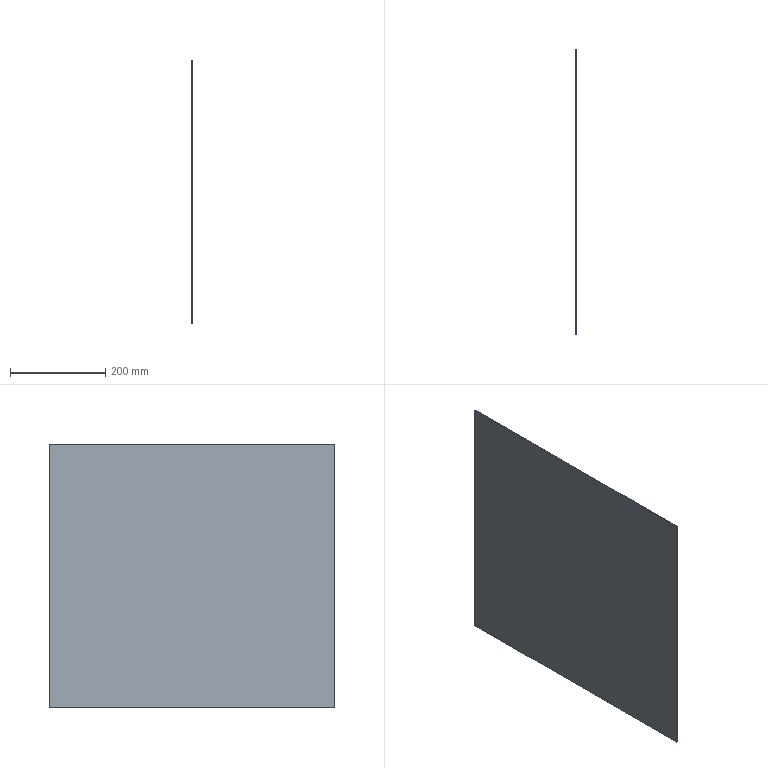Part | SolidWorks | features FlatPattern 1, SMBaseFlange 1, SheetMetal 1 | 1 solid | 6 faces | box 2 x 600 x 554 mm | volume 664800 mm3 | plane 6
STEP:
#1=CARTESIAN_POINT('',(0.,-300.,-277.));
#2=VERTEX_POINT('',#1);
#3=CARTESIAN_POINT('',(0.,300.,-277.));
#4=VERTEX_POINT('',#3);
#5=CARTESIAN_POINT('',(0.,-300.,-277.));
#6=DIRECTION('',(0.,1.,0.));
#7=VECTOR('',#6,1000.);
#8=LINE('',#5,#7);
#9=EDGE_CURVE('',#2,#4,#8,.T.);
#10=ORIENTED_EDGE('',*,*,#9,.F.);
#11=CARTESIAN_POINT('',(-2.,-300.,-277.));
#12=VERTEX_POINT('',#11);
#13=CARTESIAN_POINT('',(-2.,-300.,-277.));
#14=DIRECTION('',(1.,0.,0.));
#15=VECTOR('',#14,1000.);
#16=LINE('',#13,#15);
#17=EDGE_CURVE('',#12,#2,#16,.T.);
#18=ORIENTED_EDGE('',*,*,#17,.F.);
#19=CARTESIAN_POINT('',(-2.,300.,-277.));
#20=VERTEX_POINT('',#19);
#21=CARTESIAN_POINT('',(-2.,-300.,-277.));
#22=DIRECTION('',(0.,1.,0.));
#23=VECTOR('',#22,1000.);
#24=LINE('',#21,#23);
#25=EDGE_CURVE('',#12,#20,#24,.T.);
#26=ORIENTED_EDGE('',*,*,#25,.T.);
#27=CARTESIAN_POINT('',(-2.,300.,-277.));
#28=DIRECTION('',(1.,0.,0.));
#29=VECTOR('',#28,1000.);
#30=LINE('',#27,#29);
#31=EDGE_CURVE('',#20,#4,#30,.T.);
#32=ORIENTED_EDGE('',*,*,#31,.T.);
#33=EDGE_LOOP('',(#10,#18,#26,#32));
#34=FACE_OUTER_BOUND('',#33,.T.);
#35=CARTESIAN_POINT('',(-2.,-300.,-277.));
#36=DIRECTION('',(0.,0.,-1.));
#37=DIRECTION('',(-1.,0.,0.));
#38=AXIS2_PLACEMENT_3D('',#35,#36,#37);
#39=PLANE('',#38);
#40=ADVANCED_FACE('',(#34),#39,.T.);
#41=CARTESIAN_POINT('',(0.,-300.,277.));
#42=VERTEX_POINT('',#41);
#43=CARTESIAN_POINT('',(0.,-300.,277.));
#44=DIRECTION('',(0.,0.,-1.));
#45=VECTOR('',#44,1000.);
#46=LINE('',#43,#45);
#47=EDGE_CURVE('',#42,#2,#46,.T.);
#48=ORIENTED_EDGE('',*,*,#47,.F.);
#49=CARTESIAN_POINT('',(-2.,-300.,277.));
#50=VERTEX_POINT('',#49);
#51=CARTESIAN_POINT('',(-2.,-300.,277.));
#52=DIRECTION('',(1.,0.,0.));
#53=VECTOR('',#52,1000.);
#54=LINE('',#51,#53);
#55=EDGE_CURVE('',#50,#42,#54,.T.);
#56=ORIENTED_EDGE('',*,*,#55,.F.);
#57=CARTESIAN_POINT('',(-2.,-300.,277.));
#58=DIRECTION('',(0.,0.,-1.));
#59=VECTOR('',#58,1000.);
#60=LINE('',#57,#59);
#61=EDGE_CURVE('',#50,#12,#60,.T.);
#62=ORIENTED_EDGE('',*,*,#61,.T.);
#63=ORIENTED_EDGE('',*,*,#17,.T.);
#64=EDGE_LOOP('',(#48,#56,#62,#63));
#65=FACE_OUTER_BOUND('',#64,.T.);
#66=CARTESIAN_POINT('',(-2.,-300.,277.));
#67=DIRECTION('',(0.,-1.,0.));
#68=DIRECTION('',(0.,0.,-1.));
#69=AXIS2_PLACEMENT_3D('',#66,#67,#68);
#70=PLANE('',#69);
#71=ADVANCED_FACE('',(#65),#70,.T.);
#72=CARTESIAN_POINT('',(0.,300.,277.));
#73=VERTEX_POINT('',#72);
#74=CARTESIAN_POINT('',(0.,-300.,277.));
#75=DIRECTION('',(0.,-1.,0.));
#76=VECTOR('',#75,1000.);
#77=LINE('',#74,#76);
#78=EDGE_CURVE('',#73,#42,#77,.T.);
#79=ORIENTED_EDGE('',*,*,#78,.F.);
#80=CARTESIAN_POINT('',(-2.,300.,277.));
#81=VERTEX_POINT('',#80);
#82=CARTESIAN_POINT('',(-2.,300.,277.));
#83=DIRECTION('',(1.,0.,0.));
#84=VECTOR('',#83,1000.);
#85=LINE('',#82,#84);
#86=EDGE_CURVE('',#81,#73,#85,.T.);
#87=ORIENTED_EDGE('',*,*,#86,.F.);
#88=CARTESIAN_POINT('',(-2.,-300.,277.));
#89=DIRECTION('',(0.,-1.,0.));
#90=VECTOR('',#89,1000.);
#91=LINE('',#88,#90);
#92=EDGE_CURVE('',#81,#50,#91,.T.);
#93=ORIENTED_EDGE('',*,*,#92,.T.);
#94=ORIENTED_EDGE('',*,*,#55,.T.);
#95=EDGE_LOOP('',(#79,#87,#93,#94));
#96=FACE_OUTER_BOUND('',#95,.T.);
#97=CARTESIAN_POINT('',(-2.,-300.,277.));
#98=DIRECTION('',(0.,0.,1.));
#99=DIRECTION('',(1.,0.,0.));
#100=AXIS2_PLACEMENT_3D('',#97,#98,#99);
#101=PLANE('',#100);
#102=ADVANCED_FACE('',(#96),#101,.T.);
#103=CARTESIAN_POINT('',(0.,300.,277.));
#104=DIRECTION('',(0.,0.,1.));
#105=VECTOR('',#104,1000.);
#106=LINE('',#103,#105);
#107=EDGE_CURVE('',#4,#73,#106,.T.);
#108=ORIENTED_EDGE('',*,*,#107,.F.);
#109=ORIENTED_EDGE('',*,*,#31,.F.);
#110=CARTESIAN_POINT('',(-2.,300.,277.));
#111=DIRECTION('',(0.,0.,1.));
#112=VECTOR('',#111,1000.);
#113=LINE('',#110,#112);
#114=EDGE_CURVE('',#20,#81,#113,.T.);
#115=ORIENTED_EDGE('',*,*,#114,.T.);
#116=ORIENTED_EDGE('',*,*,#86,.T.);
#117=EDGE_LOOP('',(#108,#109,#115,#116));
#118=FACE_OUTER_BOUND('',#117,.T.);
#119=CARTESIAN_POINT('',(-2.,300.,277.));
#120=DIRECTION('',(0.,1.,0.));
#121=DIRECTION('',(0.,0.,1.));
#122=AXIS2_PLACEMENT_3D('',#119,#120,#121);
#123=PLANE('',#122);
#124=ADVANCED_FACE('',(#118),#123,.T.);
#125=ORIENTED_EDGE('',*,*,#25,.F.);
#126=ORIENTED_EDGE('',*,*,#61,.F.);
#127=ORIENTED_EDGE('',*,*,#92,.F.);
#128=ORIENTED_EDGE('',*,*,#114,.F.);
#129=EDGE_LOOP('',(#125,#126,#127,#128));
#130=FACE_OUTER_BOUND('',#129,.T.);
#131=CARTESIAN_POINT('',(-2.,0.,0.));
#132=DIRECTION('',(-1.,0.,0.));
#133=DIRECTION('',(0.,0.,1.));
#134=AXIS2_PLACEMENT_3D('',#131,#132,#133);
#135=PLANE('',#134);
#136=ADVANCED_FACE('',(#130),#135,.T.);
#137=ORIENTED_EDGE('',*,*,#9,.T.);
#138=ORIENTED_EDGE('',*,*,#107,.T.);
#139=ORIENTED_EDGE('',*,*,#78,.T.);
#140=ORIENTED_EDGE('',*,*,#47,.T.);
#141=EDGE_LOOP('',(#137,#138,#139,#140));
#142=FACE_OUTER_BOUND('',#141,.T.);
#143=CARTESIAN_POINT('',(0.,0.,0.));
#144=DIRECTION('',(-1.,0.,0.));
#145=DIRECTION('',(0.,0.,1.));
#146=AXIS2_PLACEMENT_3D('',#143,#144,#145);
#147=PLANE('',#146);
#148=ADVANCED_FACE('',(#142),#147,.F.);
#149=CLOSED_SHELL('',(#40,#71,#102,#124,#136,#148));
#150=MANIFOLD_SOLID_BREP('',#149);
#151=CARTESIAN_POINT('',(0.,0.,0.));
#152=DIRECTION('',(0.,0.,1.));
#153=DIRECTION('',(1.,0.,0.));
#154=AXIS2_PLACEMENT_3D('',#151,#152,#153);
#155=(LENGTH_UNIT()NAMED_UNIT(*)SI_UNIT(.MILLI.,.METRE.));
#156=UNCERTAINTY_MEASURE_WITH_UNIT(LENGTH_MEASURE(0.00001),#155,'','');
#157=(NAMED_UNIT(*)PLANE_ANGLE_UNIT()SI_UNIT($,.RADIAN.));
#158=(NAMED_UNIT(*)SI_UNIT($,.STERADIAN.)SOLID_ANGLE_UNIT());
#159=(GEOMETRIC_REPRESENTATION_CONTEXT(3)GLOBAL_UNCERTAINTY_ASSIGNED_CONTEXT((#156))GLOBAL_UNIT_ASSIGNED_CONTEXT((#155,#157,#158))REPRESENTATION_CONTEXT('',''));
#160=ADVANCED_BREP_SHAPE_REPRESENTATION('',(#150,#154),#159);